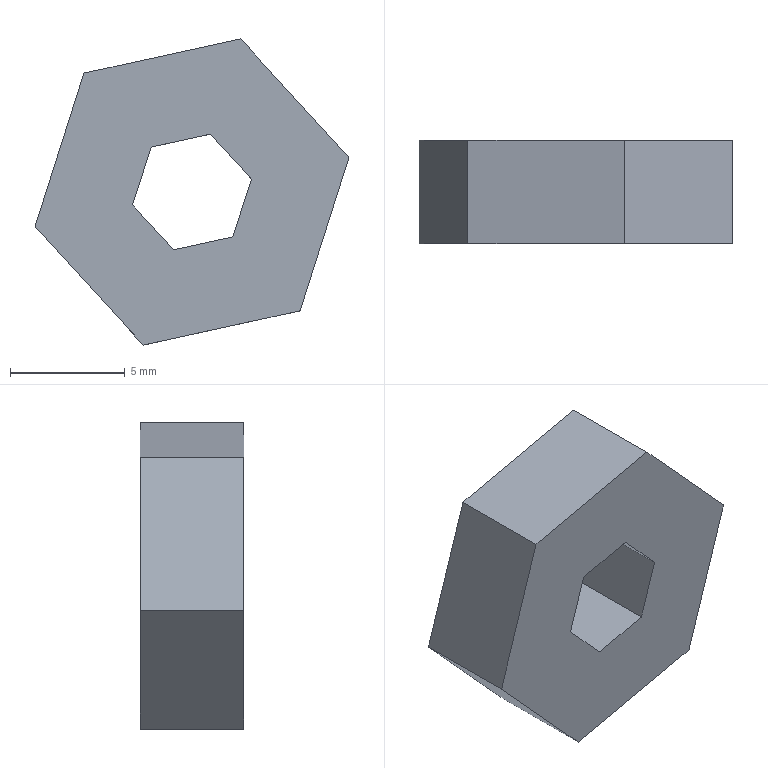Part | STEP file | Dodanie-wyci_gni_cie1_5 | 1 solid | 14 faces | box 13.678 x 4.505 x 13.341 mm | volume 491.011 mm3 | plane 14
STEP:
#1=CARTESIAN_POINT('',(0.,0.,0.));
#2=DIRECTION('',(0.,0.,1.));
#3=DIRECTION('',(1.,0.,0.));
#4=AXIS2_PLACEMENT_3D('',#1,#2,#3);
#5=CARTESIAN_POINT('',(158.921,206.145,-123.076));
#6=VERTEX_POINT('',#5);
#7=CARTESIAN_POINT('',(161.507,206.145,-122.511));
#8=VERTEX_POINT('',#7);
#9=CARTESIAN_POINT('',(158.921,206.145,-123.076));
#10=DIRECTION('',(0.977,0.00008141,0.2134));
#11=VECTOR('',#10,1.);
#12=LINE('',#9,#11);
#13=CARTESIAN_POINT('',(160.703,206.144,-125.033));
#14=DIRECTION('',(0.,-1.,0.0003815));
#15=DIRECTION('',(0.8883,-0.0001752,-0.4593));
#16=AXIS2_PLACEMENT_3D('',#13,#14,#15);
#17=PLANE('',#16);
#18=CARTESIAN_POINT('',(-2.482,0.9201));
#19=DIRECTION('',(0.7698,0.6382));
#20=VECTOR('',#19,1.);
#21=LINE('',#18,#20);
#22=(GEOMETRIC_REPRESENTATION_CONTEXT(2)PARAMETRIC_REPRESENTATION_CONTEXT()REPRESENTATION_CONTEXT('',''));
#23=DEFINITIONAL_REPRESENTATION('',(#21),#22);
#24=PCURVE('',#17,#23);
#25=CARTESIAN_POINT('',(160.214,203.895,-122.793));
#26=DIRECTION('',(0.2134,-0.0003727,-0.977));
#27=DIRECTION('',(0.977,0.00008141,0.2134));
#28=AXIS2_PLACEMENT_3D('',#25,#26,#27);
#29=PLANE('',#28);
#30=CARTESIAN_POINT('',(-1.324,-2.25));
#31=DIRECTION('',(1.,0.));
#32=VECTOR('',#31,1.);
#33=LINE('',#30,#32);
#34=(GEOMETRIC_REPRESENTATION_CONTEXT(2)PARAMETRIC_REPRESENTATION_CONTEXT()REPRESENTATION_CONTEXT('',''));
#35=DEFINITIONAL_REPRESENTATION('',(#33),#34);
#36=PCURVE('',#29,#35);
#37=SURFACE_CURVE('',#12,(#24,#36),.PCURVE_S1.);
#38=EDGE_CURVE('',#6,#8,#37,.T.);
#39=ORIENTED_EDGE('',*,*,#38,.F.);
#40=CARTESIAN_POINT('',(158.117,206.144,-125.598));
#41=VERTEX_POINT('',#40);
#42=CARTESIAN_POINT('',(158.117,206.144,-125.598));
#43=DIRECTION('',(0.3037,0.0003635,0.9528));
#44=VECTOR('',#43,1.);
#45=LINE('',#42,#44);
#46=CARTESIAN_POINT('',(-2.038,-1.69));
#47=DIRECTION('',(-0.1678,0.9858));
#48=VECTOR('',#47,1.);
#49=LINE('',#46,#48);
#50=(GEOMETRIC_REPRESENTATION_CONTEXT(2)PARAMETRIC_REPRESENTATION_CONTEXT()REPRESENTATION_CONTEXT('',''));
#51=DEFINITIONAL_REPRESENTATION('',(#49),#50);
#52=PCURVE('',#17,#51);
#53=CARTESIAN_POINT('',(158.519,203.894,-124.336));
#54=DIRECTION('',(0.9528,-0.0001158,-0.3037));
#55=DIRECTION('',(0.3037,0.0003635,0.9528));
#56=AXIS2_PLACEMENT_3D('',#53,#54,#55);
#57=PLANE('',#56);
#58=CARTESIAN_POINT('',(-1.324,-2.25));
#59=DIRECTION('',(1.,0.));
#60=VECTOR('',#59,1.);
#61=LINE('',#58,#60);
#62=(GEOMETRIC_REPRESENTATION_CONTEXT(2)PARAMETRIC_REPRESENTATION_CONTEXT()REPRESENTATION_CONTEXT('',''));
#63=DEFINITIONAL_REPRESENTATION('',(#61),#62);
#64=PCURVE('',#57,#63);
#65=SURFACE_CURVE('',#45,(#52,#64),.PCURVE_S1.);
#66=EDGE_CURVE('',#41,#6,#65,.T.);
#67=ORIENTED_EDGE('',*,*,#66,.F.);
#68=CARTESIAN_POINT('',(159.899,206.143,-127.555));
#69=VERTEX_POINT('',#68);
#70=CARTESIAN_POINT('',(159.899,206.143,-127.555));
#71=DIRECTION('',(-0.6733,0.0002821,0.7394));
#72=VECTOR('',#71,1.);
#73=LINE('',#70,#72);
#74=CARTESIAN_POINT('',(0.4442,-2.61));
#75=DIRECTION('',(-0.9377,0.3476));
#76=VECTOR('',#75,1.);
#77=LINE('',#74,#76);
#78=(GEOMETRIC_REPRESENTATION_CONTEXT(2)PARAMETRIC_REPRESENTATION_CONTEXT()REPRESENTATION_CONTEXT('',''));
#79=DEFINITIONAL_REPRESENTATION('',(#77),#78);
#80=PCURVE('',#17,#79);
#81=CARTESIAN_POINT('',(159.008,203.893,-126.576));
#82=DIRECTION('',(0.7394,0.0002568,0.6733));
#83=DIRECTION('',(-0.6733,0.0002821,0.7394));
#84=AXIS2_PLACEMENT_3D('',#81,#82,#83);
#85=PLANE('',#84);
#86=CARTESIAN_POINT('',(-1.324,-2.25));
#87=DIRECTION('',(1.,0.));
#88=VECTOR('',#87,1.);
#89=LINE('',#86,#88);
#90=(GEOMETRIC_REPRESENTATION_CONTEXT(2)PARAMETRIC_REPRESENTATION_CONTEXT()REPRESENTATION_CONTEXT('',''));
#91=DEFINITIONAL_REPRESENTATION('',(#89),#90);
#92=PCURVE('',#85,#91);
#93=SURFACE_CURVE('',#73,(#80,#92),.PCURVE_S1.);
#94=EDGE_CURVE('',#69,#41,#93,.T.);
#95=ORIENTED_EDGE('',*,*,#94,.F.);
#96=CARTESIAN_POINT('',(162.485,206.143,-126.99));
#97=VERTEX_POINT('',#96);
#98=CARTESIAN_POINT('',(162.485,206.143,-126.99));
#99=DIRECTION('',(-0.977,-0.00008141,-0.2134));
#100=VECTOR('',#99,1.);
#101=LINE('',#98,#100);
#102=CARTESIAN_POINT('',(2.482,-0.9201));
#103=DIRECTION('',(-0.7698,-0.6382));
#104=VECTOR('',#103,1.);
#105=LINE('',#102,#104);
#106=(GEOMETRIC_REPRESENTATION_CONTEXT(2)PARAMETRIC_REPRESENTATION_CONTEXT()REPRESENTATION_CONTEXT('',''));
#107=DEFINITIONAL_REPRESENTATION('',(#105),#106);
#108=PCURVE('',#17,#107);
#109=CARTESIAN_POINT('',(161.192,203.893,-127.272));
#110=DIRECTION('',(-0.2134,0.0003727,0.977));
#111=DIRECTION('',(-0.977,-0.00008141,-0.2134));
#112=AXIS2_PLACEMENT_3D('',#109,#110,#111);
#113=PLANE('',#112);
#114=CARTESIAN_POINT('',(-1.324,-2.25));
#115=DIRECTION('',(1.,0.));
#116=VECTOR('',#115,1.);
#117=LINE('',#114,#116);
#118=(GEOMETRIC_REPRESENTATION_CONTEXT(2)PARAMETRIC_REPRESENTATION_CONTEXT()REPRESENTATION_CONTEXT('',''));
#119=DEFINITIONAL_REPRESENTATION('',(#117),#118);
#120=PCURVE('',#113,#119);
#121=SURFACE_CURVE('',#101,(#108,#120),.PCURVE_S1.);
#122=EDGE_CURVE('',#97,#69,#121,.T.);
#123=ORIENTED_EDGE('',*,*,#122,.F.);
#124=CARTESIAN_POINT('',(163.289,206.144,-124.468));
#125=VERTEX_POINT('',#124);
#126=CARTESIAN_POINT('',(163.289,206.144,-124.468));
#127=DIRECTION('',(-0.3037,-0.0003635,-0.9528));
#128=VECTOR('',#127,1.);
#129=LINE('',#126,#128);
#130=CARTESIAN_POINT('',(2.038,1.69));
#131=DIRECTION('',(0.1678,-0.9858));
#132=VECTOR('',#131,1.);
#133=LINE('',#130,#132);
#134=(GEOMETRIC_REPRESENTATION_CONTEXT(2)PARAMETRIC_REPRESENTATION_CONTEXT()REPRESENTATION_CONTEXT('',''));
#135=DEFINITIONAL_REPRESENTATION('',(#133),#134);
#136=PCURVE('',#17,#135);
#137=CARTESIAN_POINT('',(162.887,203.894,-125.728));
#138=DIRECTION('',(-0.9528,0.0001158,0.3037));
#139=DIRECTION('',(-0.3037,-0.0003635,-0.9528));
#140=AXIS2_PLACEMENT_3D('',#137,#138,#139);
#141=PLANE('',#140);
#142=CARTESIAN_POINT('',(-1.324,-2.25));
#143=DIRECTION('',(1.,0.));
#144=VECTOR('',#143,1.);
#145=LINE('',#142,#144);
#146=(GEOMETRIC_REPRESENTATION_CONTEXT(2)PARAMETRIC_REPRESENTATION_CONTEXT()REPRESENTATION_CONTEXT('',''));
#147=DEFINITIONAL_REPRESENTATION('',(#145),#146);
#148=PCURVE('',#141,#147);
#149=SURFACE_CURVE('',#129,(#136,#148),.PCURVE_S1.);
#150=EDGE_CURVE('',#125,#97,#149,.T.);
#151=ORIENTED_EDGE('',*,*,#150,.F.);
#152=CARTESIAN_POINT('',(161.507,206.145,-122.511));
#153=DIRECTION('',(0.6733,-0.0002821,-0.7394));
#154=VECTOR('',#153,1.);
#155=LINE('',#152,#154);
#156=CARTESIAN_POINT('',(-0.4442,2.61));
#157=DIRECTION('',(0.9377,-0.3476));
#158=VECTOR('',#157,1.);
#159=LINE('',#156,#158);
#160=(GEOMETRIC_REPRESENTATION_CONTEXT(2)PARAMETRIC_REPRESENTATION_CONTEXT()REPRESENTATION_CONTEXT('',''));
#161=DEFINITIONAL_REPRESENTATION('',(#159),#160);
#162=PCURVE('',#17,#161);
#163=CARTESIAN_POINT('',(162.398,203.895,-123.489));
#164=DIRECTION('',(-0.7394,-0.0002568,-0.6733));
#165=DIRECTION('',(0.6733,-0.0002821,-0.7394));
#166=AXIS2_PLACEMENT_3D('',#163,#164,#165);
#167=PLANE('',#166);
#168=CARTESIAN_POINT('',(-1.324,-2.25));
#169=DIRECTION('',(1.,0.));
#170=VECTOR('',#169,1.);
#171=LINE('',#168,#170);
#172=(GEOMETRIC_REPRESENTATION_CONTEXT(2)PARAMETRIC_REPRESENTATION_CONTEXT()REPRESENTATION_CONTEXT('',''));
#173=DEFINITIONAL_REPRESENTATION('',(#171),#172);
#174=PCURVE('',#167,#173);
#175=SURFACE_CURVE('',#155,(#162,#174),.PCURVE_S1.);
#176=EDGE_CURVE('',#8,#125,#175,.T.);
#177=ORIENTED_EDGE('',*,*,#176,.F.);
#178=EDGE_LOOP('',(#39,#67,#95,#123,#151,#177));
#179=FACE_BOUND('',#178,.T.);
#180=CARTESIAN_POINT('',(158.577,206.141,-131.703));
#181=VERTEX_POINT('',#180);
#182=CARTESIAN_POINT('',(165.416,206.142,-130.209));
#183=VERTEX_POINT('',#182);
#184=CARTESIAN_POINT('',(158.577,206.141,-131.703));
#185=DIRECTION('',(0.977,0.00008141,0.2134));
#186=VECTOR('',#185,1.);
#187=LINE('',#184,#186);
#188=CARTESIAN_POINT('',(1.175,-6.901));
#189=DIRECTION('',(0.7698,0.6382));
#190=VECTOR('',#189,1.);
#191=LINE('',#188,#190);
#192=(GEOMETRIC_REPRESENTATION_CONTEXT(2)PARAMETRIC_REPRESENTATION_CONTEXT()REPRESENTATION_CONTEXT('',''));
#193=DEFINITIONAL_REPRESENTATION('',(#191),#192);
#194=PCURVE('',#17,#193);
#195=CARTESIAN_POINT('',(161.997,203.892,-130.955));
#196=DIRECTION('',(-0.2134,0.0003727,0.977));
#197=DIRECTION('',(-0.977,-0.00008141,-0.2134));
#198=AXIS2_PLACEMENT_3D('',#195,#196,#197);
#199=PLANE('',#198);
#200=CARTESIAN_POINT('',(3.5,-2.25));
#201=DIRECTION('',(-1.,0.));
#202=VECTOR('',#201,1.);
#203=LINE('',#200,#202);
#204=(GEOMETRIC_REPRESENTATION_CONTEXT(2)PARAMETRIC_REPRESENTATION_CONTEXT()REPRESENTATION_CONTEXT('',''));
#205=DEFINITIONAL_REPRESENTATION('',(#203),#204);
#206=PCURVE('',#199,#205);
#207=SURFACE_CURVE('',#187,(#194,#206),.PCURVE_S1.);
#208=EDGE_CURVE('',#181,#183,#207,.T.);
#209=ORIENTED_EDGE('',*,*,#208,.F.);
#210=CARTESIAN_POINT('',(153.864,206.143,-126.527));
#211=VERTEX_POINT('',#210);
#212=CARTESIAN_POINT('',(153.864,206.143,-126.527));
#213=DIRECTION('',(0.6733,-0.0002821,-0.7394));
#214=VECTOR('',#213,1.);
#215=LINE('',#212,#214);
#216=CARTESIAN_POINT('',(-5.389,-4.468));
#217=DIRECTION('',(0.9377,-0.3476));
#218=VECTOR('',#217,1.);
#219=LINE('',#216,#218);
#220=(GEOMETRIC_REPRESENTATION_CONTEXT(2)PARAMETRIC_REPRESENTATION_CONTEXT()REPRESENTATION_CONTEXT('',''));
#221=DEFINITIONAL_REPRESENTATION('',(#219),#220);
#222=PCURVE('',#17,#221);
#223=CARTESIAN_POINT('',(156.221,203.892,-129.114));
#224=DIRECTION('',(0.7394,0.0002568,0.6733));
#225=DIRECTION('',(-0.6733,0.0002821,0.7394));
#226=AXIS2_PLACEMENT_3D('',#223,#224,#225);
#227=PLANE('',#226);
#228=CARTESIAN_POINT('',(3.5,-2.25));
#229=DIRECTION('',(-1.,0.));
#230=VECTOR('',#229,1.);
#231=LINE('',#228,#230);
#232=(GEOMETRIC_REPRESENTATION_CONTEXT(2)PARAMETRIC_REPRESENTATION_CONTEXT()REPRESENTATION_CONTEXT('',''));
#233=DEFINITIONAL_REPRESENTATION('',(#231),#232);
#234=PCURVE('',#227,#233);
#235=SURFACE_CURVE('',#215,(#222,#234),.PCURVE_S1.);
#236=EDGE_CURVE('',#211,#181,#235,.T.);
#237=ORIENTED_EDGE('',*,*,#236,.F.);
#238=CARTESIAN_POINT('',(155.99,206.146,-119.857));
#239=VERTEX_POINT('',#238);
#240=CARTESIAN_POINT('',(155.99,206.146,-119.857));
#241=DIRECTION('',(-0.3037,-0.0003635,-0.9528));
#242=VECTOR('',#241,1.);
#243=LINE('',#240,#242);
#244=CARTESIAN_POINT('',(-6.564,2.433));
#245=DIRECTION('',(0.1678,-0.9858));
#246=VECTOR('',#245,1.);
#247=LINE('',#244,#246);
#248=(GEOMETRIC_REPRESENTATION_CONTEXT(2)PARAMETRIC_REPRESENTATION_CONTEXT()REPRESENTATION_CONTEXT('',''));
#249=DEFINITIONAL_REPRESENTATION('',(#247),#248);
#250=PCURVE('',#17,#249);
#251=CARTESIAN_POINT('',(154.927,203.895,-123.191));
#252=DIRECTION('',(0.9528,-0.0001158,-0.3037));
#253=DIRECTION('',(0.3037,0.0003635,0.9528));
#254=AXIS2_PLACEMENT_3D('',#251,#252,#253);
#255=PLANE('',#254);
#256=CARTESIAN_POINT('',(3.5,-2.25));
#257=DIRECTION('',(-1.,0.));
#258=VECTOR('',#257,1.);
#259=LINE('',#256,#258);
#260=(GEOMETRIC_REPRESENTATION_CONTEXT(2)PARAMETRIC_REPRESENTATION_CONTEXT()REPRESENTATION_CONTEXT('',''));
#261=DEFINITIONAL_REPRESENTATION('',(#259),#260);
#262=PCURVE('',#255,#261);
#263=SURFACE_CURVE('',#243,(#250,#262),.PCURVE_S1.);
#264=EDGE_CURVE('',#239,#211,#263,.T.);
#265=ORIENTED_EDGE('',*,*,#264,.F.);
#266=CARTESIAN_POINT('',(162.829,206.146,-118.363));
#267=VERTEX_POINT('',#266);
#268=CARTESIAN_POINT('',(162.829,206.146,-118.363));
#269=DIRECTION('',(-0.977,-0.00008141,-0.2134));
#270=VECTOR('',#269,1.);
#271=LINE('',#268,#270);
#272=CARTESIAN_POINT('',(-1.175,6.901));
#273=DIRECTION('',(-0.7698,-0.6382));
#274=VECTOR('',#273,1.);
#275=LINE('',#272,#274);
#276=(GEOMETRIC_REPRESENTATION_CONTEXT(2)PARAMETRIC_REPRESENTATION_CONTEXT()REPRESENTATION_CONTEXT('',''));
#277=DEFINITIONAL_REPRESENTATION('',(#275),#276);
#278=PCURVE('',#17,#277);
#279=CARTESIAN_POINT('',(159.409,203.896,-119.109));
#280=DIRECTION('',(0.2134,-0.0003727,-0.977));
#281=DIRECTION('',(0.977,0.00008141,0.2134));
#282=AXIS2_PLACEMENT_3D('',#279,#280,#281);
#283=PLANE('',#282);
#284=CARTESIAN_POINT('',(3.5,-2.25));
#285=DIRECTION('',(-1.,0.));
#286=VECTOR('',#285,1.);
#287=LINE('',#284,#286);
#288=(GEOMETRIC_REPRESENTATION_CONTEXT(2)PARAMETRIC_REPRESENTATION_CONTEXT()REPRESENTATION_CONTEXT('',''));
#289=DEFINITIONAL_REPRESENTATION('',(#287),#288);
#290=PCURVE('',#283,#289);
#291=SURFACE_CURVE('',#271,(#278,#290),.PCURVE_S1.);
#292=EDGE_CURVE('',#267,#239,#291,.T.);
#293=ORIENTED_EDGE('',*,*,#292,.F.);
#294=CARTESIAN_POINT('',(167.542,206.145,-123.539));
#295=VERTEX_POINT('',#294);
#296=CARTESIAN_POINT('',(167.542,206.145,-123.539));
#297=DIRECTION('',(-0.6733,0.0002821,0.7394));
#298=VECTOR('',#297,1.);
#299=LINE('',#296,#298);
#300=CARTESIAN_POINT('',(5.389,4.468));
#301=DIRECTION('',(-0.9377,0.3476));
#302=VECTOR('',#301,1.);
#303=LINE('',#300,#302);
#304=(GEOMETRIC_REPRESENTATION_CONTEXT(2)PARAMETRIC_REPRESENTATION_CONTEXT()REPRESENTATION_CONTEXT('',''));
#305=DEFINITIONAL_REPRESENTATION('',(#303),#304);
#306=PCURVE('',#17,#305);
#307=CARTESIAN_POINT('',(165.186,203.895,-120.95));
#308=DIRECTION('',(-0.7394,-0.0002568,-0.6733));
#309=DIRECTION('',(0.6733,-0.0002821,-0.7394));
#310=AXIS2_PLACEMENT_3D('',#307,#308,#309);
#311=PLANE('',#310);
#312=CARTESIAN_POINT('',(3.5,-2.25));
#313=DIRECTION('',(-1.,0.));
#314=VECTOR('',#313,1.);
#315=LINE('',#312,#314);
#316=(GEOMETRIC_REPRESENTATION_CONTEXT(2)PARAMETRIC_REPRESENTATION_CONTEXT()REPRESENTATION_CONTEXT('',''));
#317=DEFINITIONAL_REPRESENTATION('',(#315),#316);
#318=PCURVE('',#311,#317);
#319=SURFACE_CURVE('',#299,(#306,#318),.PCURVE_S1.);
#320=EDGE_CURVE('',#295,#267,#319,.T.);
#321=ORIENTED_EDGE('',*,*,#320,.F.);
#322=CARTESIAN_POINT('',(165.416,206.142,-130.209));
#323=DIRECTION('',(0.3037,0.0003635,0.9528));
#324=VECTOR('',#323,1.);
#325=LINE('',#322,#324);
#326=CARTESIAN_POINT('',(6.564,-2.433));
#327=DIRECTION('',(-0.1678,0.9858));
#328=VECTOR('',#327,1.);
#329=LINE('',#326,#328);
#330=(GEOMETRIC_REPRESENTATION_CONTEXT(2)PARAMETRIC_REPRESENTATION_CONTEXT()REPRESENTATION_CONTEXT('',''));
#331=DEFINITIONAL_REPRESENTATION('',(#329),#330);
#332=PCURVE('',#17,#331);
#333=CARTESIAN_POINT('',(166.479,203.893,-126.873));
#334=DIRECTION('',(-0.9528,0.0001158,0.3037));
#335=DIRECTION('',(-0.3037,-0.0003635,-0.9528));
#336=AXIS2_PLACEMENT_3D('',#333,#334,#335);
#337=PLANE('',#336);
#338=CARTESIAN_POINT('',(3.5,-2.25));
#339=DIRECTION('',(-1.,0.));
#340=VECTOR('',#339,1.);
#341=LINE('',#338,#340);
#342=(GEOMETRIC_REPRESENTATION_CONTEXT(2)PARAMETRIC_REPRESENTATION_CONTEXT()REPRESENTATION_CONTEXT('',''));
#343=DEFINITIONAL_REPRESENTATION('',(#341),#342);
#344=PCURVE('',#337,#343);
#345=SURFACE_CURVE('',#325,(#332,#344),.PCURVE_S1.);
#346=EDGE_CURVE('',#183,#295,#345,.T.);
#347=ORIENTED_EDGE('',*,*,#346,.F.);
#348=EDGE_LOOP('',(#209,#237,#265,#293,#321,#347));
#349=FACE_BOUND('',#348,.T.);
#350=ADVANCED_FACE('',(#179,#349),#17,.F.);
#351=CARTESIAN_POINT('',(163.289,201.644,-124.466));
#352=VERTEX_POINT('',#351);
#353=CARTESIAN_POINT('',(161.507,201.645,-122.509));
#354=VERTEX_POINT('',#353);
#355=CARTESIAN_POINT('',(163.289,201.644,-124.466));
#356=DIRECTION('',(-0.6733,0.0002821,0.7394));
#357=VECTOR('',#356,1.);
#358=LINE('',#355,#357);
#359=CARTESIAN_POINT('',(1.324,2.25));
#360=DIRECTION('',(-1.,0.));
#361=VECTOR('',#360,1.);
#362=LINE('',#359,#361);
#363=(GEOMETRIC_REPRESENTATION_CONTEXT(2)PARAMETRIC_REPRESENTATION_CONTEXT()REPRESENTATION_CONTEXT('',''));
#364=DEFINITIONAL_REPRESENTATION('',(#362),#363);
#365=PCURVE('',#167,#364);
#366=CARTESIAN_POINT('',(160.703,201.644,-125.031));
#367=DIRECTION('',(0.,-1.,0.0003815));
#368=DIRECTION('',(0.8883,-0.0001752,-0.4593));
#369=AXIS2_PLACEMENT_3D('',#366,#367,#368);
#370=PLANE('',#369);
#371=CARTESIAN_POINT('',(2.038,1.69));
#372=DIRECTION('',(-0.9377,0.3476));
#373=VECTOR('',#372,1.);
#374=LINE('',#371,#373);
#375=(GEOMETRIC_REPRESENTATION_CONTEXT(2)PARAMETRIC_REPRESENTATION_CONTEXT()REPRESENTATION_CONTEXT('',''));
#376=DEFINITIONAL_REPRESENTATION('',(#374),#375);
#377=PCURVE('',#370,#376);
#378=SURFACE_CURVE('',#358,(#365,#377),.PCURVE_S1.);
#379=EDGE_CURVE('',#352,#354,#378,.T.);
#380=ORIENTED_EDGE('',*,*,#379,.T.);
#381=CARTESIAN_POINT('',(161.507,201.645,-122.509));
#382=DIRECTION('',(0.,1.,-0.0003815));
#383=VECTOR('',#382,1.);
#384=LINE('',#381,#383);
#385=CARTESIAN_POINT('',(-1.324,2.25));
#386=DIRECTION('',(0.,-1.));
#387=VECTOR('',#386,1.);
#388=LINE('',#385,#387);
#389=(GEOMETRIC_REPRESENTATION_CONTEXT(2)PARAMETRIC_REPRESENTATION_CONTEXT()REPRESENTATION_CONTEXT('',''));
#390=DEFINITIONAL_REPRESENTATION('',(#388),#389);
#391=PCURVE('',#167,#390);
#392=CARTESIAN_POINT('',(1.324,2.25));
#393=DIRECTION('',(0.,-1.));
#394=VECTOR('',#393,1.);
#395=LINE('',#392,#394);
#396=(GEOMETRIC_REPRESENTATION_CONTEXT(2)PARAMETRIC_REPRESENTATION_CONTEXT()REPRESENTATION_CONTEXT('',''));
#397=DEFINITIONAL_REPRESENTATION('',(#395),#396);
#398=PCURVE('',#29,#397);
#399=SURFACE_CURVE('',#384,(#391,#398),.PCURVE_S1.);
#400=EDGE_CURVE('',#354,#8,#399,.T.);
#401=ORIENTED_EDGE('',*,*,#400,.T.);
#402=ORIENTED_EDGE('',*,*,#176,.T.);
#403=CARTESIAN_POINT('',(163.289,206.144,-124.468));
#404=DIRECTION('',(0.,-1.,0.0003815));
#405=VECTOR('',#404,1.);
#406=LINE('',#403,#405);
#407=CARTESIAN_POINT('',(1.324,-2.25));
#408=DIRECTION('',(0.,1.));
#409=VECTOR('',#408,1.);
#410=LINE('',#407,#409);
#411=(GEOMETRIC_REPRESENTATION_CONTEXT(2)PARAMETRIC_REPRESENTATION_CONTEXT()REPRESENTATION_CONTEXT('',''));
#412=DEFINITIONAL_REPRESENTATION('',(#410),#411);
#413=PCURVE('',#167,#412);
#414=CARTESIAN_POINT('',(-1.324,-2.25));
#415=DIRECTION('',(0.,1.));
#416=VECTOR('',#415,1.);
#417=LINE('',#414,#416);
#418=(GEOMETRIC_REPRESENTATION_CONTEXT(2)PARAMETRIC_REPRESENTATION_CONTEXT()REPRESENTATION_CONTEXT('',''));
#419=DEFINITIONAL_REPRESENTATION('',(#417),#418);
#420=PCURVE('',#141,#419);
#421=SURFACE_CURVE('',#406,(#413,#420),.PCURVE_S1.);
#422=EDGE_CURVE('',#125,#352,#421,.T.);
#423=ORIENTED_EDGE('',*,*,#422,.T.);
#424=EDGE_LOOP('',(#380,#401,#402,#423));
#425=FACE_BOUND('',#424,.T.);
#426=ADVANCED_FACE('',(#425),#167,.T.);
#427=CARTESIAN_POINT('',(158.921,201.645,-123.074));
#428=VERTEX_POINT('',#427);
#429=CARTESIAN_POINT('',(161.507,201.645,-122.509));
#430=DIRECTION('',(-0.977,-0.00008141,-0.2134));
#431=VECTOR('',#430,1.);
#432=LINE('',#429,#431);
#433=CARTESIAN_POINT('',(1.324,2.25));
#434=DIRECTION('',(-1.,0.));
#435=VECTOR('',#434,1.);
#436=LINE('',#433,#435);
#437=(GEOMETRIC_REPRESENTATION_CONTEXT(2)PARAMETRIC_REPRESENTATION_CONTEXT()REPRESENTATION_CONTEXT('',''));
#438=DEFINITIONAL_REPRESENTATION('',(#436),#437);
#439=PCURVE('',#29,#438);
#440=CARTESIAN_POINT('',(-0.4442,2.61));
#441=DIRECTION('',(-0.7698,-0.6382));
#442=VECTOR('',#441,1.);
#443=LINE('',#440,#442);
#444=(GEOMETRIC_REPRESENTATION_CONTEXT(2)PARAMETRIC_REPRESENTATION_CONTEXT()REPRESENTATION_CONTEXT('',''));
#445=DEFINITIONAL_REPRESENTATION('',(#443),#444);
#446=PCURVE('',#370,#445);
#447=SURFACE_CURVE('',#432,(#439,#446),.PCURVE_S1.);
#448=EDGE_CURVE('',#354,#428,#447,.T.);
#449=ORIENTED_EDGE('',*,*,#448,.T.);
#450=CARTESIAN_POINT('',(158.921,201.645,-123.074));
#451=DIRECTION('',(0.,1.,-0.0003815));
#452=VECTOR('',#451,1.);
#453=LINE('',#450,#452);
#454=CARTESIAN_POINT('',(-1.324,2.25));
#455=DIRECTION('',(0.,-1.));
#456=VECTOR('',#455,1.);
#457=LINE('',#454,#456);
#458=(GEOMETRIC_REPRESENTATION_CONTEXT(2)PARAMETRIC_REPRESENTATION_CONTEXT()REPRESENTATION_CONTEXT('',''));
#459=DEFINITIONAL_REPRESENTATION('',(#457),#458);
#460=PCURVE('',#29,#459);
#461=CARTESIAN_POINT('',(1.324,2.25));
#462=DIRECTION('',(0.,-1.));
#463=VECTOR('',#462,1.);
#464=LINE('',#461,#463);
#465=(GEOMETRIC_REPRESENTATION_CONTEXT(2)PARAMETRIC_REPRESENTATION_CONTEXT()REPRESENTATION_CONTEXT('',''));
#466=DEFINITIONAL_REPRESENTATION('',(#464),#465);
#467=PCURVE('',#57,#466);
#468=SURFACE_CURVE('',#453,(#460,#467),.PCURVE_S1.);
#469=EDGE_CURVE('',#428,#6,#468,.T.);
#470=ORIENTED_EDGE('',*,*,#469,.T.);
#471=ORIENTED_EDGE('',*,*,#38,.T.);
#472=ORIENTED_EDGE('',*,*,#400,.F.);
#473=EDGE_LOOP('',(#449,#470,#471,#472));
#474=FACE_BOUND('',#473,.T.);
#475=ADVANCED_FACE('',(#474),#29,.T.);
#476=CARTESIAN_POINT('',(158.117,201.644,-125.596));
#477=VERTEX_POINT('',#476);
#478=CARTESIAN_POINT('',(158.921,201.645,-123.074));
#479=DIRECTION('',(-0.3037,-0.0003635,-0.9528));
#480=VECTOR('',#479,1.);
#481=LINE('',#478,#480);
#482=CARTESIAN_POINT('',(1.324,2.25));
#483=DIRECTION('',(-1.,0.));
#484=VECTOR('',#483,1.);
#485=LINE('',#482,#484);
#486=(GEOMETRIC_REPRESENTATION_CONTEXT(2)PARAMETRIC_REPRESENTATION_CONTEXT()REPRESENTATION_CONTEXT('',''));
#487=DEFINITIONAL_REPRESENTATION('',(#485),#486);
#488=PCURVE('',#57,#487);
#489=CARTESIAN_POINT('',(-2.482,0.9201));
#490=DIRECTION('',(0.1678,-0.9858));
#491=VECTOR('',#490,1.);
#492=LINE('',#489,#491);
#493=(GEOMETRIC_REPRESENTATION_CONTEXT(2)PARAMETRIC_REPRESENTATION_CONTEXT()REPRESENTATION_CONTEXT('',''));
#494=DEFINITIONAL_REPRESENTATION('',(#492),#493);
#495=PCURVE('',#370,#494);
#496=SURFACE_CURVE('',#481,(#488,#495),.PCURVE_S1.);
#497=EDGE_CURVE('',#428,#477,#496,.T.);
#498=ORIENTED_EDGE('',*,*,#497,.T.);
#499=CARTESIAN_POINT('',(158.117,201.644,-125.596));
#500=DIRECTION('',(0.,1.,-0.0003815));
#501=VECTOR('',#500,1.);
#502=LINE('',#499,#501);
#503=CARTESIAN_POINT('',(-1.324,2.25));
#504=DIRECTION('',(0.,-1.));
#505=VECTOR('',#504,1.);
#506=LINE('',#503,#505);
#507=(GEOMETRIC_REPRESENTATION_CONTEXT(2)PARAMETRIC_REPRESENTATION_CONTEXT()REPRESENTATION_CONTEXT('',''));
#508=DEFINITIONAL_REPRESENTATION('',(#506),#507);
#509=PCURVE('',#57,#508);
#510=CARTESIAN_POINT('',(1.324,2.25));
#511=DIRECTION('',(0.,-1.));
#512=VECTOR('',#511,1.);
#513=LINE('',#510,#512);
#514=(GEOMETRIC_REPRESENTATION_CONTEXT(2)PARAMETRIC_REPRESENTATION_CONTEXT()REPRESENTATION_CONTEXT('',''));
#515=DEFINITIONAL_REPRESENTATION('',(#513),#514);
#516=PCURVE('',#85,#515);
#517=SURFACE_CURVE('',#502,(#509,#516),.PCURVE_S1.);
#518=EDGE_CURVE('',#477,#41,#517,.T.);
#519=ORIENTED_EDGE('',*,*,#518,.T.);
#520=ORIENTED_EDGE('',*,*,#66,.T.);
#521=ORIENTED_EDGE('',*,*,#469,.F.);
#522=EDGE_LOOP('',(#498,#519,#520,#521));
#523=FACE_BOUND('',#522,.T.);
#524=ADVANCED_FACE('',(#523),#57,.T.);
#525=CARTESIAN_POINT('',(159.899,201.643,-127.554));
#526=VERTEX_POINT('',#525);
#527=CARTESIAN_POINT('',(158.117,201.644,-125.596));
#528=DIRECTION('',(0.6733,-0.0002821,-0.7394));
#529=VECTOR('',#528,1.);
#530=LINE('',#527,#529);
#531=CARTESIAN_POINT('',(1.324,2.25));
#532=DIRECTION('',(-1.,0.));
#533=VECTOR('',#532,1.);
#534=LINE('',#531,#533);
#535=(GEOMETRIC_REPRESENTATION_CONTEXT(2)PARAMETRIC_REPRESENTATION_CONTEXT()REPRESENTATION_CONTEXT('',''));
#536=DEFINITIONAL_REPRESENTATION('',(#534),#535);
#537=PCURVE('',#85,#536);
#538=CARTESIAN_POINT('',(-2.038,-1.69));
#539=DIRECTION('',(0.9377,-0.3476));
#540=VECTOR('',#539,1.);
#541=LINE('',#538,#540);
#542=(GEOMETRIC_REPRESENTATION_CONTEXT(2)PARAMETRIC_REPRESENTATION_CONTEXT()REPRESENTATION_CONTEXT('',''));
#543=DEFINITIONAL_REPRESENTATION('',(#541),#542);
#544=PCURVE('',#370,#543);
#545=SURFACE_CURVE('',#530,(#537,#544),.PCURVE_S1.);
#546=EDGE_CURVE('',#477,#526,#545,.T.);
#547=ORIENTED_EDGE('',*,*,#546,.T.);
#548=CARTESIAN_POINT('',(159.899,201.643,-127.554));
#549=DIRECTION('',(0.,1.,-0.0003815));
#550=VECTOR('',#549,1.);
#551=LINE('',#548,#550);
#552=CARTESIAN_POINT('',(-1.324,2.25));
#553=DIRECTION('',(0.,-1.));
#554=VECTOR('',#553,1.);
#555=LINE('',#552,#554);
#556=(GEOMETRIC_REPRESENTATION_CONTEXT(2)PARAMETRIC_REPRESENTATION_CONTEXT()REPRESENTATION_CONTEXT('',''));
#557=DEFINITIONAL_REPRESENTATION('',(#555),#556);
#558=PCURVE('',#85,#557);
#559=CARTESIAN_POINT('',(1.324,2.25));
#560=DIRECTION('',(0.,-1.));
#561=VECTOR('',#560,1.);
#562=LINE('',#559,#561);
#563=(GEOMETRIC_REPRESENTATION_CONTEXT(2)PARAMETRIC_REPRESENTATION_CONTEXT()REPRESENTATION_CONTEXT('',''));
#564=DEFINITIONAL_REPRESENTATION('',(#562),#563);
#565=PCURVE('',#113,#564);
#566=SURFACE_CURVE('',#551,(#558,#565),.PCURVE_S1.);
#567=EDGE_CURVE('',#526,#69,#566,.T.);
#568=ORIENTED_EDGE('',*,*,#567,.T.);
#569=ORIENTED_EDGE('',*,*,#94,.T.);
#570=ORIENTED_EDGE('',*,*,#518,.F.);
#571=EDGE_LOOP('',(#547,#568,#569,#570));
#572=FACE_BOUND('',#571,.T.);
#573=ADVANCED_FACE('',(#572),#85,.T.);
#574=CARTESIAN_POINT('',(162.485,201.643,-126.989));
#575=VERTEX_POINT('',#574);
#576=CARTESIAN_POINT('',(159.899,201.643,-127.554));
#577=DIRECTION('',(0.977,0.00008141,0.2134));
#578=VECTOR('',#577,1.);
#579=LINE('',#576,#578);
#580=CARTESIAN_POINT('',(1.324,2.25));
#581=DIRECTION('',(-1.,0.));
#582=VECTOR('',#581,1.);
#583=LINE('',#580,#582);
#584=(GEOMETRIC_REPRESENTATION_CONTEXT(2)PARAMETRIC_REPRESENTATION_CONTEXT()REPRESENTATION_CONTEXT('',''));
#585=DEFINITIONAL_REPRESENTATION('',(#583),#584);
#586=PCURVE('',#113,#585);
#587=CARTESIAN_POINT('',(0.4442,-2.61));
#588=DIRECTION('',(0.7698,0.6382));
#589=VECTOR('',#588,1.);
#590=LINE('',#587,#589);
#591=(GEOMETRIC_REPRESENTATION_CONTEXT(2)PARAMETRIC_REPRESENTATION_CONTEXT()REPRESENTATION_CONTEXT('',''));
#592=DEFINITIONAL_REPRESENTATION('',(#590),#591);
#593=PCURVE('',#370,#592);
#594=SURFACE_CURVE('',#579,(#586,#593),.PCURVE_S1.);
#595=EDGE_CURVE('',#526,#575,#594,.T.);
#596=ORIENTED_EDGE('',*,*,#595,.T.);
#597=CARTESIAN_POINT('',(162.485,201.643,-126.989));
#598=DIRECTION('',(0.,1.,-0.0003815));
#599=VECTOR('',#598,1.);
#600=LINE('',#597,#599);
#601=CARTESIAN_POINT('',(-1.324,2.25));
#602=DIRECTION('',(0.,-1.));
#603=VECTOR('',#602,1.);
#604=LINE('',#601,#603);
#605=(GEOMETRIC_REPRESENTATION_CONTEXT(2)PARAMETRIC_REPRESENTATION_CONTEXT()REPRESENTATION_CONTEXT('',''));
#606=DEFINITIONAL_REPRESENTATION('',(#604),#605);
#607=PCURVE('',#113,#606);
#608=CARTESIAN_POINT('',(1.324,2.25));
#609=DIRECTION('',(0.,-1.));
#610=VECTOR('',#609,1.);
#611=LINE('',#608,#610);
#612=(GEOMETRIC_REPRESENTATION_CONTEXT(2)PARAMETRIC_REPRESENTATION_CONTEXT()REPRESENTATION_CONTEXT('',''));
#613=DEFINITIONAL_REPRESENTATION('',(#611),#612);
#614=PCURVE('',#141,#613);
#615=SURFACE_CURVE('',#600,(#607,#614),.PCURVE_S1.);
#616=EDGE_CURVE('',#575,#97,#615,.T.);
#617=ORIENTED_EDGE('',*,*,#616,.T.);
#618=ORIENTED_EDGE('',*,*,#122,.T.);
#619=ORIENTED_EDGE('',*,*,#567,.F.);
#620=EDGE_LOOP('',(#596,#617,#618,#619));
#621=FACE_BOUND('',#620,.T.);
#622=ADVANCED_FACE('',(#621),#113,.T.);
#623=CARTESIAN_POINT('',(162.485,201.643,-126.989));
#624=DIRECTION('',(0.3037,0.0003635,0.9528));
#625=VECTOR('',#624,1.);
#626=LINE('',#623,#625);
#627=CARTESIAN_POINT('',(1.324,2.25));
#628=DIRECTION('',(-1.,0.));
#629=VECTOR('',#628,1.);
#630=LINE('',#627,#629);
#631=(GEOMETRIC_REPRESENTATION_CONTEXT(2)PARAMETRIC_REPRESENTATION_CONTEXT()REPRESENTATION_CONTEXT('',''));
#632=DEFINITIONAL_REPRESENTATION('',(#630),#631);
#633=PCURVE('',#141,#632);
#634=CARTESIAN_POINT('',(2.482,-0.9201));
#635=DIRECTION('',(-0.1678,0.9858));
#636=VECTOR('',#635,1.);
#637=LINE('',#634,#636);
#638=(GEOMETRIC_REPRESENTATION_CONTEXT(2)PARAMETRIC_REPRESENTATION_CONTEXT()REPRESENTATION_CONTEXT('',''));
#639=DEFINITIONAL_REPRESENTATION('',(#637),#638);
#640=PCURVE('',#370,#639);
#641=SURFACE_CURVE('',#626,(#633,#640),.PCURVE_S1.);
#642=EDGE_CURVE('',#575,#352,#641,.T.);
#643=ORIENTED_EDGE('',*,*,#642,.T.);
#644=ORIENTED_EDGE('',*,*,#422,.F.);
#645=ORIENTED_EDGE('',*,*,#150,.T.);
#646=ORIENTED_EDGE('',*,*,#616,.F.);
#647=EDGE_LOOP('',(#643,#644,#645,#646));
#648=FACE_BOUND('',#647,.T.);
#649=ADVANCED_FACE('',(#648),#141,.T.);
#650=CARTESIAN_POINT('',(167.542,201.645,-123.537));
#651=VERTEX_POINT('',#650);
#652=CARTESIAN_POINT('',(167.542,201.645,-123.537));
#653=DIRECTION('',(0.,1.,-0.0003815));
#654=VECTOR('',#653,1.);
#655=LINE('',#652,#654);
#656=CARTESIAN_POINT('',(-3.5,2.25));
#657=DIRECTION('',(0.,-1.));
#658=VECTOR('',#657,1.);
#659=LINE('',#656,#658);
#660=(GEOMETRIC_REPRESENTATION_CONTEXT(2)PARAMETRIC_REPRESENTATION_CONTEXT()REPRESENTATION_CONTEXT('',''));
#661=DEFINITIONAL_REPRESENTATION('',(#659),#660);
#662=PCURVE('',#337,#661);
#663=CARTESIAN_POINT('',(3.5,2.25));
#664=DIRECTION('',(0.,-1.));
#665=VECTOR('',#664,1.);
#666=LINE('',#663,#665);
#667=(GEOMETRIC_REPRESENTATION_CONTEXT(2)PARAMETRIC_REPRESENTATION_CONTEXT()REPRESENTATION_CONTEXT('',''));
#668=DEFINITIONAL_REPRESENTATION('',(#666),#667);
#669=PCURVE('',#311,#668);
#670=SURFACE_CURVE('',#655,(#662,#669),.PCURVE_S1.);
#671=EDGE_CURVE('',#651,#295,#670,.T.);
#672=ORIENTED_EDGE('',*,*,#671,.F.);
#673=CARTESIAN_POINT('',(165.416,201.642,-130.207));
#674=VERTEX_POINT('',#673);
#675=CARTESIAN_POINT('',(165.416,201.642,-130.207));
#676=DIRECTION('',(0.3037,0.0003635,0.9528));
#677=VECTOR('',#676,1.);
#678=LINE('',#675,#677);
#679=CARTESIAN_POINT('',(3.5,2.25));
#680=DIRECTION('',(-1.,0.));
#681=VECTOR('',#680,1.);
#682=LINE('',#679,#681);
#683=(GEOMETRIC_REPRESENTATION_CONTEXT(2)PARAMETRIC_REPRESENTATION_CONTEXT()REPRESENTATION_CONTEXT('',''));
#684=DEFINITIONAL_REPRESENTATION('',(#682),#683);
#685=PCURVE('',#337,#684);
#686=CARTESIAN_POINT('',(6.564,-2.433));
#687=DIRECTION('',(-0.1678,0.9858));
#688=VECTOR('',#687,1.);
#689=LINE('',#686,#688);
#690=(GEOMETRIC_REPRESENTATION_CONTEXT(2)PARAMETRIC_REPRESENTATION_CONTEXT()REPRESENTATION_CONTEXT('',''));
#691=DEFINITIONAL_REPRESENTATION('',(#689),#690);
#692=PCURVE('',#370,#691);
#693=SURFACE_CURVE('',#678,(#685,#692),.PCURVE_S1.);
#694=EDGE_CURVE('',#674,#651,#693,.T.);
#695=ORIENTED_EDGE('',*,*,#694,.F.);
#696=CARTESIAN_POINT('',(165.416,206.142,-130.209));
#697=DIRECTION('',(0.,-1.,0.0003815));
#698=VECTOR('',#697,1.);
#699=LINE('',#696,#698);
#700=CARTESIAN_POINT('',(3.5,-2.25));
#701=DIRECTION('',(0.,1.));
#702=VECTOR('',#701,1.);
#703=LINE('',#700,#702);
#704=(GEOMETRIC_REPRESENTATION_CONTEXT(2)PARAMETRIC_REPRESENTATION_CONTEXT()REPRESENTATION_CONTEXT('',''));
#705=DEFINITIONAL_REPRESENTATION('',(#703),#704);
#706=PCURVE('',#337,#705);
#707=CARTESIAN_POINT('',(-3.5,-2.25));
#708=DIRECTION('',(0.,1.));
#709=VECTOR('',#708,1.);
#710=LINE('',#707,#709);
#711=(GEOMETRIC_REPRESENTATION_CONTEXT(2)PARAMETRIC_REPRESENTATION_CONTEXT()REPRESENTATION_CONTEXT('',''));
#712=DEFINITIONAL_REPRESENTATION('',(#710),#711);
#713=PCURVE('',#199,#712);
#714=SURFACE_CURVE('',#699,(#706,#713),.PCURVE_S1.);
#715=EDGE_CURVE('',#183,#674,#714,.T.);
#716=ORIENTED_EDGE('',*,*,#715,.F.);
#717=ORIENTED_EDGE('',*,*,#346,.T.);
#718=EDGE_LOOP('',(#672,#695,#716,#717));
#719=FACE_BOUND('',#718,.T.);
#720=ADVANCED_FACE('',(#719),#337,.F.);
#721=ORIENTED_EDGE('',*,*,#715,.T.);
#722=CARTESIAN_POINT('',(158.577,201.641,-131.701));
#723=VERTEX_POINT('',#722);
#724=CARTESIAN_POINT('',(158.577,201.641,-131.701));
#725=DIRECTION('',(0.977,0.00008141,0.2134));
#726=VECTOR('',#725,1.);
#727=LINE('',#724,#726);
#728=CARTESIAN_POINT('',(3.5,2.25));
#729=DIRECTION('',(-1.,0.));
#730=VECTOR('',#729,1.);
#731=LINE('',#728,#730);
#732=(GEOMETRIC_REPRESENTATION_CONTEXT(2)PARAMETRIC_REPRESENTATION_CONTEXT()REPRESENTATION_CONTEXT('',''));
#733=DEFINITIONAL_REPRESENTATION('',(#731),#732);
#734=PCURVE('',#199,#733);
#735=CARTESIAN_POINT('',(1.175,-6.901));
#736=DIRECTION('',(0.7698,0.6382));
#737=VECTOR('',#736,1.);
#738=LINE('',#735,#737);
#739=(GEOMETRIC_REPRESENTATION_CONTEXT(2)PARAMETRIC_REPRESENTATION_CONTEXT()REPRESENTATION_CONTEXT('',''));
#740=DEFINITIONAL_REPRESENTATION('',(#738),#739);
#741=PCURVE('',#370,#740);
#742=SURFACE_CURVE('',#727,(#734,#741),.PCURVE_S1.);
#743=EDGE_CURVE('',#723,#674,#742,.T.);
#744=ORIENTED_EDGE('',*,*,#743,.F.);
#745=CARTESIAN_POINT('',(158.577,206.141,-131.703));
#746=DIRECTION('',(0.,-1.,0.0003815));
#747=VECTOR('',#746,1.);
#748=LINE('',#745,#747);
#749=CARTESIAN_POINT('',(3.5,-2.25));
#750=DIRECTION('',(0.,1.));
#751=VECTOR('',#750,1.);
#752=LINE('',#749,#751);
#753=(GEOMETRIC_REPRESENTATION_CONTEXT(2)PARAMETRIC_REPRESENTATION_CONTEXT()REPRESENTATION_CONTEXT('',''));
#754=DEFINITIONAL_REPRESENTATION('',(#752),#753);
#755=PCURVE('',#199,#754);
#756=CARTESIAN_POINT('',(-3.5,-2.25));
#757=DIRECTION('',(0.,1.));
#758=VECTOR('',#757,1.);
#759=LINE('',#756,#758);
#760=(GEOMETRIC_REPRESENTATION_CONTEXT(2)PARAMETRIC_REPRESENTATION_CONTEXT()REPRESENTATION_CONTEXT('',''));
#761=DEFINITIONAL_REPRESENTATION('',(#759),#760);
#762=PCURVE('',#227,#761);
#763=SURFACE_CURVE('',#748,(#755,#762),.PCURVE_S1.);
#764=EDGE_CURVE('',#181,#723,#763,.T.);
#765=ORIENTED_EDGE('',*,*,#764,.F.);
#766=ORIENTED_EDGE('',*,*,#208,.T.);
#767=EDGE_LOOP('',(#721,#744,#765,#766));
#768=FACE_BOUND('',#767,.T.);
#769=ADVANCED_FACE('',(#768),#199,.F.);
#770=ORIENTED_EDGE('',*,*,#764,.T.);
#771=CARTESIAN_POINT('',(153.864,201.643,-126.525));
#772=VERTEX_POINT('',#771);
#773=CARTESIAN_POINT('',(153.864,201.643,-126.525));
#774=DIRECTION('',(0.6733,-0.0002821,-0.7394));
#775=VECTOR('',#774,1.);
#776=LINE('',#773,#775);
#777=CARTESIAN_POINT('',(3.5,2.25));
#778=DIRECTION('',(-1.,0.));
#779=VECTOR('',#778,1.);
#780=LINE('',#777,#779);
#781=(GEOMETRIC_REPRESENTATION_CONTEXT(2)PARAMETRIC_REPRESENTATION_CONTEXT()REPRESENTATION_CONTEXT('',''));
#782=DEFINITIONAL_REPRESENTATION('',(#780),#781);
#783=PCURVE('',#227,#782);
#784=CARTESIAN_POINT('',(-5.389,-4.468));
#785=DIRECTION('',(0.9377,-0.3476));
#786=VECTOR('',#785,1.);
#787=LINE('',#784,#786);
#788=(GEOMETRIC_REPRESENTATION_CONTEXT(2)PARAMETRIC_REPRESENTATION_CONTEXT()REPRESENTATION_CONTEXT('',''));
#789=DEFINITIONAL_REPRESENTATION('',(#787),#788);
#790=PCURVE('',#370,#789);
#791=SURFACE_CURVE('',#776,(#783,#790),.PCURVE_S1.);
#792=EDGE_CURVE('',#772,#723,#791,.T.);
#793=ORIENTED_EDGE('',*,*,#792,.F.);
#794=CARTESIAN_POINT('',(153.864,206.143,-126.527));
#795=DIRECTION('',(0.,-1.,0.0003815));
#796=VECTOR('',#795,1.);
#797=LINE('',#794,#796);
#798=CARTESIAN_POINT('',(3.5,-2.25));
#799=DIRECTION('',(0.,1.));
#800=VECTOR('',#799,1.);
#801=LINE('',#798,#800);
#802=(GEOMETRIC_REPRESENTATION_CONTEXT(2)PARAMETRIC_REPRESENTATION_CONTEXT()REPRESENTATION_CONTEXT('',''));
#803=DEFINITIONAL_REPRESENTATION('',(#801),#802);
#804=PCURVE('',#227,#803);
#805=CARTESIAN_POINT('',(-3.5,-2.25));
#806=DIRECTION('',(0.,1.));
#807=VECTOR('',#806,1.);
#808=LINE('',#805,#807);
#809=(GEOMETRIC_REPRESENTATION_CONTEXT(2)PARAMETRIC_REPRESENTATION_CONTEXT()REPRESENTATION_CONTEXT('',''));
#810=DEFINITIONAL_REPRESENTATION('',(#808),#809);
#811=PCURVE('',#255,#810);
#812=SURFACE_CURVE('',#797,(#804,#811),.PCURVE_S1.);
#813=EDGE_CURVE('',#211,#772,#812,.T.);
#814=ORIENTED_EDGE('',*,*,#813,.F.);
#815=ORIENTED_EDGE('',*,*,#236,.T.);
#816=EDGE_LOOP('',(#770,#793,#814,#815));
#817=FACE_BOUND('',#816,.T.);
#818=ADVANCED_FACE('',(#817),#227,.F.);
#819=ORIENTED_EDGE('',*,*,#813,.T.);
#820=CARTESIAN_POINT('',(155.99,201.646,-119.855));
#821=VERTEX_POINT('',#820);
#822=CARTESIAN_POINT('',(155.99,201.646,-119.855));
#823=DIRECTION('',(-0.3037,-0.0003635,-0.9528));
#824=VECTOR('',#823,1.);
#825=LINE('',#822,#824);
#826=CARTESIAN_POINT('',(3.5,2.25));
#827=DIRECTION('',(-1.,0.));
#828=VECTOR('',#827,1.);
#829=LINE('',#826,#828);
#830=(GEOMETRIC_REPRESENTATION_CONTEXT(2)PARAMETRIC_REPRESENTATION_CONTEXT()REPRESENTATION_CONTEXT('',''));
#831=DEFINITIONAL_REPRESENTATION('',(#829),#830);
#832=PCURVE('',#255,#831);
#833=CARTESIAN_POINT('',(-6.564,2.433));
#834=DIRECTION('',(0.1678,-0.9858));
#835=VECTOR('',#834,1.);
#836=LINE('',#833,#835);
#837=(GEOMETRIC_REPRESENTATION_CONTEXT(2)PARAMETRIC_REPRESENTATION_CONTEXT()REPRESENTATION_CONTEXT('',''));
#838=DEFINITIONAL_REPRESENTATION('',(#836),#837);
#839=PCURVE('',#370,#838);
#840=SURFACE_CURVE('',#825,(#832,#839),.PCURVE_S1.);
#841=EDGE_CURVE('',#821,#772,#840,.T.);
#842=ORIENTED_EDGE('',*,*,#841,.F.);
#843=CARTESIAN_POINT('',(155.99,206.146,-119.857));
#844=DIRECTION('',(0.,-1.,0.0003815));
#845=VECTOR('',#844,1.);
#846=LINE('',#843,#845);
#847=CARTESIAN_POINT('',(3.5,-2.25));
#848=DIRECTION('',(0.,1.));
#849=VECTOR('',#848,1.);
#850=LINE('',#847,#849);
#851=(GEOMETRIC_REPRESENTATION_CONTEXT(2)PARAMETRIC_REPRESENTATION_CONTEXT()REPRESENTATION_CONTEXT('',''));
#852=DEFINITIONAL_REPRESENTATION('',(#850),#851);
#853=PCURVE('',#255,#852);
#854=CARTESIAN_POINT('',(-3.5,-2.25));
#855=DIRECTION('',(0.,1.));
#856=VECTOR('',#855,1.);
#857=LINE('',#854,#856);
#858=(GEOMETRIC_REPRESENTATION_CONTEXT(2)PARAMETRIC_REPRESENTATION_CONTEXT()REPRESENTATION_CONTEXT('',''));
#859=DEFINITIONAL_REPRESENTATION('',(#857),#858);
#860=PCURVE('',#283,#859);
#861=SURFACE_CURVE('',#846,(#853,#860),.PCURVE_S1.);
#862=EDGE_CURVE('',#239,#821,#861,.T.);
#863=ORIENTED_EDGE('',*,*,#862,.F.);
#864=ORIENTED_EDGE('',*,*,#264,.T.);
#865=EDGE_LOOP('',(#819,#842,#863,#864));
#866=FACE_BOUND('',#865,.T.);
#867=ADVANCED_FACE('',(#866),#255,.F.);
#868=ORIENTED_EDGE('',*,*,#862,.T.);
#869=CARTESIAN_POINT('',(162.829,201.646,-118.362));
#870=VERTEX_POINT('',#869);
#871=CARTESIAN_POINT('',(162.829,201.646,-118.362));
#872=DIRECTION('',(-0.977,-0.00008141,-0.2134));
#873=VECTOR('',#872,1.);
#874=LINE('',#871,#873);
#875=CARTESIAN_POINT('',(3.5,2.25));
#876=DIRECTION('',(-1.,0.));
#877=VECTOR('',#876,1.);
#878=LINE('',#875,#877);
#879=(GEOMETRIC_REPRESENTATION_CONTEXT(2)PARAMETRIC_REPRESENTATION_CONTEXT()REPRESENTATION_CONTEXT('',''));
#880=DEFINITIONAL_REPRESENTATION('',(#878),#879);
#881=PCURVE('',#283,#880);
#882=CARTESIAN_POINT('',(-1.175,6.901));
#883=DIRECTION('',(-0.7698,-0.6382));
#884=VECTOR('',#883,1.);
#885=LINE('',#882,#884);
#886=(GEOMETRIC_REPRESENTATION_CONTEXT(2)PARAMETRIC_REPRESENTATION_CONTEXT()REPRESENTATION_CONTEXT('',''));
#887=DEFINITIONAL_REPRESENTATION('',(#885),#886);
#888=PCURVE('',#370,#887);
#889=SURFACE_CURVE('',#874,(#881,#888),.PCURVE_S1.);
#890=EDGE_CURVE('',#870,#821,#889,.T.);
#891=ORIENTED_EDGE('',*,*,#890,.F.);
#892=CARTESIAN_POINT('',(162.829,206.146,-118.363));
#893=DIRECTION('',(0.,-1.,0.0003815));
#894=VECTOR('',#893,1.);
#895=LINE('',#892,#894);
#896=CARTESIAN_POINT('',(3.5,-2.25));
#897=DIRECTION('',(0.,1.));
#898=VECTOR('',#897,1.);
#899=LINE('',#896,#898);
#900=(GEOMETRIC_REPRESENTATION_CONTEXT(2)PARAMETRIC_REPRESENTATION_CONTEXT()REPRESENTATION_CONTEXT('',''));
#901=DEFINITIONAL_REPRESENTATION('',(#899),#900);
#902=PCURVE('',#283,#901);
#903=CARTESIAN_POINT('',(-3.5,-2.25));
#904=DIRECTION('',(0.,1.));
#905=VECTOR('',#904,1.);
#906=LINE('',#903,#905);
#907=(GEOMETRIC_REPRESENTATION_CONTEXT(2)PARAMETRIC_REPRESENTATION_CONTEXT()REPRESENTATION_CONTEXT('',''));
#908=DEFINITIONAL_REPRESENTATION('',(#906),#907);
#909=PCURVE('',#311,#908);
#910=SURFACE_CURVE('',#895,(#902,#909),.PCURVE_S1.);
#911=EDGE_CURVE('',#267,#870,#910,.T.);
#912=ORIENTED_EDGE('',*,*,#911,.F.);
#913=ORIENTED_EDGE('',*,*,#292,.T.);
#914=EDGE_LOOP('',(#868,#891,#912,#913));
#915=FACE_BOUND('',#914,.T.);
#916=ADVANCED_FACE('',(#915),#283,.F.);
#917=ORIENTED_EDGE('',*,*,#911,.T.);
#918=CARTESIAN_POINT('',(167.542,201.645,-123.537));
#919=DIRECTION('',(-0.6733,0.0002821,0.7394));
#920=VECTOR('',#919,1.);
#921=LINE('',#918,#920);
#922=CARTESIAN_POINT('',(3.5,2.25));
#923=DIRECTION('',(-1.,0.));
#924=VECTOR('',#923,1.);
#925=LINE('',#922,#924);
#926=(GEOMETRIC_REPRESENTATION_CONTEXT(2)PARAMETRIC_REPRESENTATION_CONTEXT()REPRESENTATION_CONTEXT('',''));
#927=DEFINITIONAL_REPRESENTATION('',(#925),#926);
#928=PCURVE('',#311,#927);
#929=CARTESIAN_POINT('',(5.389,4.468));
#930=DIRECTION('',(-0.9377,0.3476));
#931=VECTOR('',#930,1.);
#932=LINE('',#929,#931);
#933=(GEOMETRIC_REPRESENTATION_CONTEXT(2)PARAMETRIC_REPRESENTATION_CONTEXT()REPRESENTATION_CONTEXT('',''));
#934=DEFINITIONAL_REPRESENTATION('',(#932),#933);
#935=PCURVE('',#370,#934);
#936=SURFACE_CURVE('',#921,(#928,#935),.PCURVE_S1.);
#937=EDGE_CURVE('',#651,#870,#936,.T.);
#938=ORIENTED_EDGE('',*,*,#937,.F.);
#939=ORIENTED_EDGE('',*,*,#671,.T.);
#940=ORIENTED_EDGE('',*,*,#320,.T.);
#941=EDGE_LOOP('',(#917,#938,#939,#940));
#942=FACE_BOUND('',#941,.T.);
#943=ADVANCED_FACE('',(#942),#311,.F.);
#944=ORIENTED_EDGE('',*,*,#546,.F.);
#945=ORIENTED_EDGE('',*,*,#497,.F.);
#946=ORIENTED_EDGE('',*,*,#448,.F.);
#947=ORIENTED_EDGE('',*,*,#379,.F.);
#948=ORIENTED_EDGE('',*,*,#642,.F.);
#949=ORIENTED_EDGE('',*,*,#595,.F.);
#950=EDGE_LOOP('',(#944,#945,#946,#947,#948,#949));
#951=FACE_BOUND('',#950,.T.);
#952=ORIENTED_EDGE('',*,*,#792,.T.);
#953=ORIENTED_EDGE('',*,*,#743,.T.);
#954=ORIENTED_EDGE('',*,*,#694,.T.);
#955=ORIENTED_EDGE('',*,*,#937,.T.);
#956=ORIENTED_EDGE('',*,*,#890,.T.);
#957=ORIENTED_EDGE('',*,*,#841,.T.);
#958=EDGE_LOOP('',(#952,#953,#954,#955,#956,#957));
#959=FACE_BOUND('',#958,.T.);
#960=ADVANCED_FACE('',(#951,#959),#370,.T.);
#961=CLOSED_SHELL('',(#350,#426,#475,#524,#573,#622,#649,#720,#769,#818,#867,#916,#943,#960));
#962=MANIFOLD_SOLID_BREP('',#961);
#963=(LENGTH_UNIT()NAMED_UNIT(*)SI_UNIT(.MILLI.,.METRE.));
#964=UNCERTAINTY_MEASURE_WITH_UNIT(LENGTH_MEASURE(0.0000001),#963,'','');
#965=(NAMED_UNIT(*)PLANE_ANGLE_UNIT()SI_UNIT($,.RADIAN.));
#966=(NAMED_UNIT(*)SI_UNIT($,.STERADIAN.)SOLID_ANGLE_UNIT());
#967=(GEOMETRIC_REPRESENTATION_CONTEXT(3)GLOBAL_UNCERTAINTY_ASSIGNED_CONTEXT((#964))GLOBAL_UNIT_ASSIGNED_CONTEXT((#963,#965,#966))REPRESENTATION_CONTEXT('',''));
#968=ADVANCED_BREP_SHAPE_REPRESENTATION('',(#4,#962),#967);